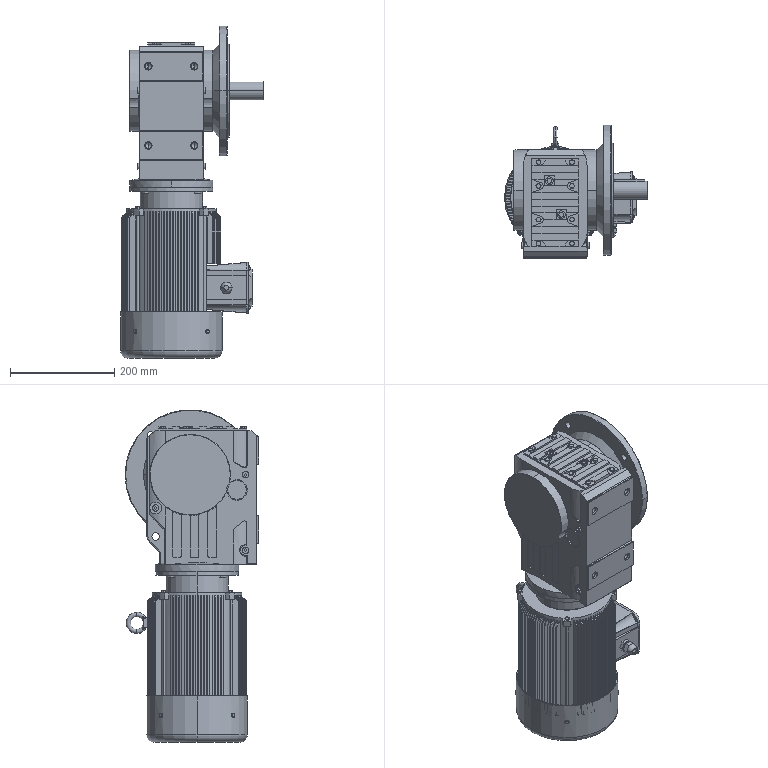Part | SolidWorks | 4 solids | 1717 faces | box 274.5 x 257 x 638 mm | volume 13749904 mm3 | plane 856 | cylinder 434 | cone 274 | torus 137 | sphere 8 | spline 8 | commonest cylinder face diameters 190.357 x167 4 x35 2 x23 171.786 x23 14.4 x22 12.4 x12